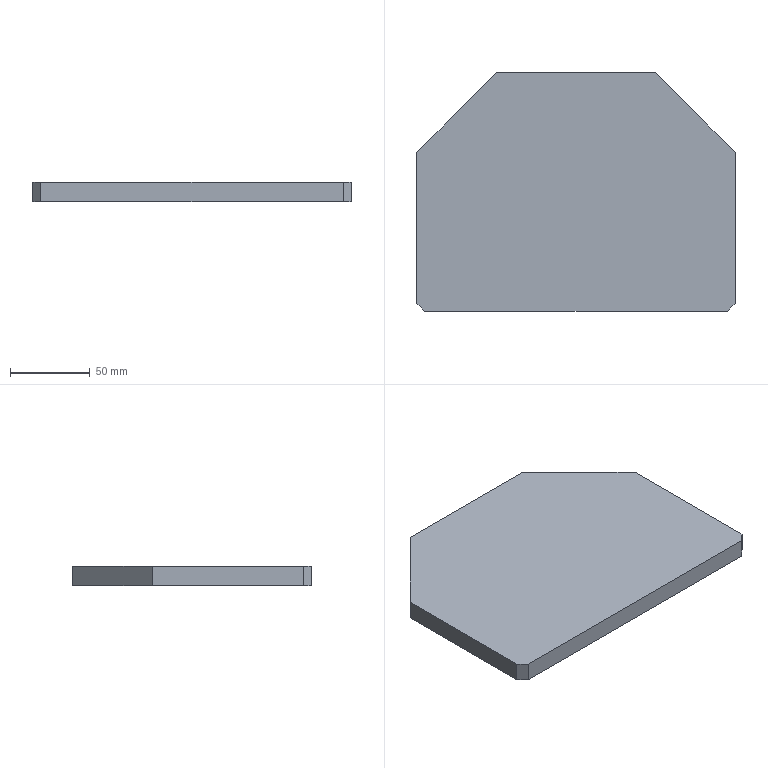Part | STEP file | [15] | 1 solid | 10 faces | box 200 x 150 x 12 mm | volume 329700 mm3 | plane 10
STEP:
#1=CARTESIAN_POINT('',(0.,0.,0.));
#2=DIRECTION('',(0.,0.,1.));
#3=DIRECTION('',(1.,0.,0.));
#4=AXIS2_PLACEMENT_3D('',#1,#2,#3);
#5=CARTESIAN_POINT('',(200.,5.,0.));
#6=VERTEX_POINT('',#5);
#7=CARTESIAN_POINT('',(200.,100.,0.));
#8=VERTEX_POINT('',#7);
#9=CARTESIAN_POINT('',(200.,75.,0.));
#10=DIRECTION('',(0.,1.,0.));
#11=VECTOR('',#10,1.);
#12=LINE('',#9,#11);
#13=CARTESIAN_POINT('',(100.,75.,0.));
#14=DIRECTION('',(0.,0.,-1.));
#15=DIRECTION('',(0.,-1.,0.));
#16=AXIS2_PLACEMENT_3D('',#13,#14,#15);
#17=PLANE('',#16);
#18=CARTESIAN_POINT('',(0.,-100.));
#19=DIRECTION('',(-1.,0.));
#20=VECTOR('',#19,1.);
#21=LINE('',#18,#20);
#22=(GEOMETRIC_REPRESENTATION_CONTEXT(2)PARAMETRIC_REPRESENTATION_CONTEXT()REPRESENTATION_CONTEXT('',''));
#23=DEFINITIONAL_REPRESENTATION('',(#21),#22);
#24=PCURVE('',#17,#23);
#25=CARTESIAN_POINT('',(200.,75.,12.));
#26=DIRECTION('',(1.,0.,0.));
#27=DIRECTION('',(0.,0.,1.));
#28=AXIS2_PLACEMENT_3D('',#25,#26,#27);
#29=PLANE('',#28);
#30=CARTESIAN_POINT('',(-12.,0.));
#31=DIRECTION('',(0.,-1.));
#32=VECTOR('',#31,1.);
#33=LINE('',#30,#32);
#34=(GEOMETRIC_REPRESENTATION_CONTEXT(2)PARAMETRIC_REPRESENTATION_CONTEXT()REPRESENTATION_CONTEXT('',''));
#35=DEFINITIONAL_REPRESENTATION('',(#33),#34);
#36=PCURVE('',#29,#35);
#37=SURFACE_CURVE('',#12,(#24,#36),.PCURVE_S1.);
#38=EDGE_CURVE('',#6,#8,#37,.T.);
#39=ORIENTED_EDGE('',*,*,#38,.F.);
#40=CARTESIAN_POINT('',(195.,0.,0.));
#41=VERTEX_POINT('',#40);
#42=CARTESIAN_POINT('',(185.,-10.,0.));
#43=DIRECTION('',(-0.7071,-0.7071,0.));
#44=VECTOR('',#43,1.);
#45=LINE('',#42,#44);
#46=CARTESIAN_POINT('',(85.,-85.));
#47=DIRECTION('',(0.7071,0.7071));
#48=VECTOR('',#47,1.);
#49=LINE('',#46,#48);
#50=(GEOMETRIC_REPRESENTATION_CONTEXT(2)PARAMETRIC_REPRESENTATION_CONTEXT()REPRESENTATION_CONTEXT('',''));
#51=DEFINITIONAL_REPRESENTATION('',(#49),#50);
#52=PCURVE('',#17,#51);
#53=CARTESIAN_POINT('',(200.,5.,12.));
#54=DIRECTION('',(-0.7071,0.7071,0.));
#55=DIRECTION('',(0.,0.,-1.));
#56=AXIS2_PLACEMENT_3D('',#53,#54,#55);
#57=PLANE('',#56);
#58=CARTESIAN_POINT('',(12.,21.213));
#59=DIRECTION('',(0.,1.));
#60=VECTOR('',#59,1.);
#61=LINE('',#58,#60);
#62=(GEOMETRIC_REPRESENTATION_CONTEXT(2)PARAMETRIC_REPRESENTATION_CONTEXT()REPRESENTATION_CONTEXT('',''));
#63=DEFINITIONAL_REPRESENTATION('',(#61),#62);
#64=PCURVE('',#57,#63);
#65=SURFACE_CURVE('',#45,(#52,#64),.PCURVE_S1.);
#66=EDGE_CURVE('',#6,#41,#65,.T.);
#67=ORIENTED_EDGE('',*,*,#66,.T.);
#68=CARTESIAN_POINT('',(5.,0.,0.));
#69=VERTEX_POINT('',#68);
#70=CARTESIAN_POINT('',(100.,0.,0.));
#71=DIRECTION('',(1.,0.,0.));
#72=VECTOR('',#71,1.);
#73=LINE('',#70,#72);
#74=CARTESIAN_POINT('',(75.,0.));
#75=DIRECTION('',(0.,-1.));
#76=VECTOR('',#75,1.);
#77=LINE('',#74,#76);
#78=(GEOMETRIC_REPRESENTATION_CONTEXT(2)PARAMETRIC_REPRESENTATION_CONTEXT()REPRESENTATION_CONTEXT('',''));
#79=DEFINITIONAL_REPRESENTATION('',(#77),#78);
#80=PCURVE('',#17,#79);
#81=CARTESIAN_POINT('',(100.,0.,12.));
#82=DIRECTION('',(0.,-1.,0.));
#83=DIRECTION('',(0.,0.,1.));
#84=AXIS2_PLACEMENT_3D('',#81,#82,#83);
#85=PLANE('',#84);
#86=CARTESIAN_POINT('',(-12.,0.));
#87=DIRECTION('',(0.,-1.));
#88=VECTOR('',#87,1.);
#89=LINE('',#86,#88);
#90=(GEOMETRIC_REPRESENTATION_CONTEXT(2)PARAMETRIC_REPRESENTATION_CONTEXT()REPRESENTATION_CONTEXT('',''));
#91=DEFINITIONAL_REPRESENTATION('',(#89),#90);
#92=PCURVE('',#85,#91);
#93=SURFACE_CURVE('',#73,(#80,#92),.PCURVE_S1.);
#94=EDGE_CURVE('',#69,#41,#93,.T.);
#95=ORIENTED_EDGE('',*,*,#94,.F.);
#96=CARTESIAN_POINT('',(0.,5.,0.));
#97=VERTEX_POINT('',#96);
#98=CARTESIAN_POINT('',(15.,-10.,0.));
#99=DIRECTION('',(-0.7071,0.7071,0.));
#100=VECTOR('',#99,1.);
#101=LINE('',#98,#100);
#102=CARTESIAN_POINT('',(85.,85.));
#103=DIRECTION('',(-0.7071,0.7071));
#104=VECTOR('',#103,1.);
#105=LINE('',#102,#104);
#106=(GEOMETRIC_REPRESENTATION_CONTEXT(2)PARAMETRIC_REPRESENTATION_CONTEXT()REPRESENTATION_CONTEXT('',''));
#107=DEFINITIONAL_REPRESENTATION('',(#105),#106);
#108=PCURVE('',#17,#107);
#109=CARTESIAN_POINT('',(5.,0.,12.));
#110=DIRECTION('',(0.7071,0.7071,0.));
#111=DIRECTION('',(0.,0.,-1.));
#112=AXIS2_PLACEMENT_3D('',#109,#110,#111);
#113=PLANE('',#112);
#114=CARTESIAN_POINT('',(12.,-14.142));
#115=DIRECTION('',(0.,1.));
#116=VECTOR('',#115,1.);
#117=LINE('',#114,#116);
#118=(GEOMETRIC_REPRESENTATION_CONTEXT(2)PARAMETRIC_REPRESENTATION_CONTEXT()REPRESENTATION_CONTEXT('',''));
#119=DEFINITIONAL_REPRESENTATION('',(#117),#118);
#120=PCURVE('',#113,#119);
#121=SURFACE_CURVE('',#101,(#108,#120),.PCURVE_S1.);
#122=EDGE_CURVE('',#69,#97,#121,.T.);
#123=ORIENTED_EDGE('',*,*,#122,.T.);
#124=CARTESIAN_POINT('',(0.,100.,0.));
#125=VERTEX_POINT('',#124);
#126=CARTESIAN_POINT('',(0.,75.,0.));
#127=DIRECTION('',(0.,-1.,0.));
#128=VECTOR('',#127,1.);
#129=LINE('',#126,#128);
#130=CARTESIAN_POINT('',(0.,100.));
#131=DIRECTION('',(1.,0.));
#132=VECTOR('',#131,1.);
#133=LINE('',#130,#132);
#134=(GEOMETRIC_REPRESENTATION_CONTEXT(2)PARAMETRIC_REPRESENTATION_CONTEXT()REPRESENTATION_CONTEXT('',''));
#135=DEFINITIONAL_REPRESENTATION('',(#133),#134);
#136=PCURVE('',#17,#135);
#137=CARTESIAN_POINT('',(0.,75.,12.));
#138=DIRECTION('',(-1.,0.,0.));
#139=DIRECTION('',(0.,0.,-1.));
#140=AXIS2_PLACEMENT_3D('',#137,#138,#139);
#141=PLANE('',#140);
#142=CARTESIAN_POINT('',(12.,0.));
#143=DIRECTION('',(0.,1.));
#144=VECTOR('',#143,1.);
#145=LINE('',#142,#144);
#146=(GEOMETRIC_REPRESENTATION_CONTEXT(2)PARAMETRIC_REPRESENTATION_CONTEXT()REPRESENTATION_CONTEXT('',''));
#147=DEFINITIONAL_REPRESENTATION('',(#145),#146);
#148=PCURVE('',#141,#147);
#149=SURFACE_CURVE('',#129,(#136,#148),.PCURVE_S1.);
#150=EDGE_CURVE('',#125,#97,#149,.T.);
#151=ORIENTED_EDGE('',*,*,#150,.F.);
#152=CARTESIAN_POINT('',(50.,150.,0.));
#153=VERTEX_POINT('',#152);
#154=CARTESIAN_POINT('',(37.5,137.5,0.));
#155=DIRECTION('',(0.7071,0.7071,0.));
#156=VECTOR('',#155,1.);
#157=LINE('',#154,#156);
#158=CARTESIAN_POINT('',(-62.5,62.5));
#159=DIRECTION('',(-0.7071,-0.7071));
#160=VECTOR('',#159,1.);
#161=LINE('',#158,#160);
#162=(GEOMETRIC_REPRESENTATION_CONTEXT(2)PARAMETRIC_REPRESENTATION_CONTEXT()REPRESENTATION_CONTEXT('',''));
#163=DEFINITIONAL_REPRESENTATION('',(#161),#162);
#164=PCURVE('',#17,#163);
#165=CARTESIAN_POINT('',(0.,100.,12.));
#166=DIRECTION('',(0.7071,-0.7071,0.));
#167=DIRECTION('',(0.,0.,-1.));
#168=AXIS2_PLACEMENT_3D('',#165,#166,#167);
#169=PLANE('',#168);
#170=CARTESIAN_POINT('',(12.,53.033));
#171=DIRECTION('',(0.,1.));
#172=VECTOR('',#171,1.);
#173=LINE('',#170,#172);
#174=(GEOMETRIC_REPRESENTATION_CONTEXT(2)PARAMETRIC_REPRESENTATION_CONTEXT()REPRESENTATION_CONTEXT('',''));
#175=DEFINITIONAL_REPRESENTATION('',(#173),#174);
#176=PCURVE('',#169,#175);
#177=SURFACE_CURVE('',#157,(#164,#176),.PCURVE_S1.);
#178=EDGE_CURVE('',#125,#153,#177,.T.);
#179=ORIENTED_EDGE('',*,*,#178,.T.);
#180=CARTESIAN_POINT('',(150.,150.,0.));
#181=VERTEX_POINT('',#180);
#182=CARTESIAN_POINT('',(100.,150.,0.));
#183=DIRECTION('',(-1.,0.,0.));
#184=VECTOR('',#183,1.);
#185=LINE('',#182,#184);
#186=CARTESIAN_POINT('',(-75.,0.));
#187=DIRECTION('',(0.,1.));
#188=VECTOR('',#187,1.);
#189=LINE('',#186,#188);
#190=(GEOMETRIC_REPRESENTATION_CONTEXT(2)PARAMETRIC_REPRESENTATION_CONTEXT()REPRESENTATION_CONTEXT('',''));
#191=DEFINITIONAL_REPRESENTATION('',(#189),#190);
#192=PCURVE('',#17,#191);
#193=CARTESIAN_POINT('',(100.,150.,12.));
#194=DIRECTION('',(0.,1.,0.));
#195=DIRECTION('',(0.,0.,-1.));
#196=AXIS2_PLACEMENT_3D('',#193,#194,#195);
#197=PLANE('',#196);
#198=CARTESIAN_POINT('',(12.,0.));
#199=DIRECTION('',(0.,1.));
#200=VECTOR('',#199,1.);
#201=LINE('',#198,#200);
#202=(GEOMETRIC_REPRESENTATION_CONTEXT(2)PARAMETRIC_REPRESENTATION_CONTEXT()REPRESENTATION_CONTEXT('',''));
#203=DEFINITIONAL_REPRESENTATION('',(#201),#202);
#204=PCURVE('',#197,#203);
#205=SURFACE_CURVE('',#185,(#192,#204),.PCURVE_S1.);
#206=EDGE_CURVE('',#181,#153,#205,.T.);
#207=ORIENTED_EDGE('',*,*,#206,.F.);
#208=CARTESIAN_POINT('',(162.5,137.5,0.));
#209=DIRECTION('',(0.7071,-0.7071,0.));
#210=VECTOR('',#209,1.);
#211=LINE('',#208,#210);
#212=CARTESIAN_POINT('',(-62.5,-62.5));
#213=DIRECTION('',(0.7071,-0.7071));
#214=VECTOR('',#213,1.);
#215=LINE('',#212,#214);
#216=(GEOMETRIC_REPRESENTATION_CONTEXT(2)PARAMETRIC_REPRESENTATION_CONTEXT()REPRESENTATION_CONTEXT('',''));
#217=DEFINITIONAL_REPRESENTATION('',(#215),#216);
#218=PCURVE('',#17,#217);
#219=CARTESIAN_POINT('',(150.,150.,12.));
#220=DIRECTION('',(-0.7071,-0.7071,0.));
#221=DIRECTION('',(0.,0.,-1.));
#222=AXIS2_PLACEMENT_3D('',#219,#220,#221);
#223=PLANE('',#222);
#224=CARTESIAN_POINT('',(12.,17.678));
#225=DIRECTION('',(0.,1.));
#226=VECTOR('',#225,1.);
#227=LINE('',#224,#226);
#228=(GEOMETRIC_REPRESENTATION_CONTEXT(2)PARAMETRIC_REPRESENTATION_CONTEXT()REPRESENTATION_CONTEXT('',''));
#229=DEFINITIONAL_REPRESENTATION('',(#227),#228);
#230=PCURVE('',#223,#229);
#231=SURFACE_CURVE('',#211,(#218,#230),.PCURVE_S1.);
#232=EDGE_CURVE('',#181,#8,#231,.T.);
#233=ORIENTED_EDGE('',*,*,#232,.T.);
#234=EDGE_LOOP('',(#39,#67,#95,#123,#151,#179,#207,#233));
#235=FACE_BOUND('',#234,.T.);
#236=ADVANCED_FACE('',(#235),#17,.T.);
#237=CARTESIAN_POINT('',(200.,100.,12.));
#238=VERTEX_POINT('',#237);
#239=CARTESIAN_POINT('',(200.,5.,12.));
#240=VERTEX_POINT('',#239);
#241=CARTESIAN_POINT('',(200.,75.,12.));
#242=DIRECTION('',(0.,-1.,0.));
#243=VECTOR('',#242,1.);
#244=LINE('',#241,#243);
#245=CARTESIAN_POINT('',(0.,0.));
#246=DIRECTION('',(0.,1.));
#247=VECTOR('',#246,1.);
#248=LINE('',#245,#247);
#249=(GEOMETRIC_REPRESENTATION_CONTEXT(2)PARAMETRIC_REPRESENTATION_CONTEXT()REPRESENTATION_CONTEXT('',''));
#250=DEFINITIONAL_REPRESENTATION('',(#248),#249);
#251=PCURVE('',#29,#250);
#252=CARTESIAN_POINT('',(100.,75.,12.));
#253=DIRECTION('',(0.,0.,1.));
#254=DIRECTION('',(0.,1.,0.));
#255=AXIS2_PLACEMENT_3D('',#252,#253,#254);
#256=PLANE('',#255);
#257=CARTESIAN_POINT('',(0.,-100.));
#258=DIRECTION('',(-1.,0.));
#259=VECTOR('',#258,1.);
#260=LINE('',#257,#259);
#261=(GEOMETRIC_REPRESENTATION_CONTEXT(2)PARAMETRIC_REPRESENTATION_CONTEXT()REPRESENTATION_CONTEXT('',''));
#262=DEFINITIONAL_REPRESENTATION('',(#260),#261);
#263=PCURVE('',#256,#262);
#264=SURFACE_CURVE('',#244,(#251,#263),.PCURVE_S1.);
#265=EDGE_CURVE('',#238,#240,#264,.T.);
#266=ORIENTED_EDGE('',*,*,#265,.T.);
#267=CARTESIAN_POINT('',(200.,5.,12.));
#268=DIRECTION('',(0.,0.,-1.));
#269=VECTOR('',#268,1.);
#270=LINE('',#267,#269);
#271=CARTESIAN_POINT('',(0.,70.));
#272=DIRECTION('',(-1.,0.));
#273=VECTOR('',#272,1.);
#274=LINE('',#271,#273);
#275=(GEOMETRIC_REPRESENTATION_CONTEXT(2)PARAMETRIC_REPRESENTATION_CONTEXT()REPRESENTATION_CONTEXT('',''));
#276=DEFINITIONAL_REPRESENTATION('',(#274),#275);
#277=PCURVE('',#29,#276);
#278=CARTESIAN_POINT('',(0.,0.));
#279=DIRECTION('',(1.,0.));
#280=VECTOR('',#279,1.);
#281=LINE('',#278,#280);
#282=(GEOMETRIC_REPRESENTATION_CONTEXT(2)PARAMETRIC_REPRESENTATION_CONTEXT()REPRESENTATION_CONTEXT('',''));
#283=DEFINITIONAL_REPRESENTATION('',(#281),#282);
#284=PCURVE('',#57,#283);
#285=SURFACE_CURVE('',#270,(#277,#284),.PCURVE_S1.);
#286=EDGE_CURVE('',#240,#6,#285,.T.);
#287=ORIENTED_EDGE('',*,*,#286,.T.);
#288=ORIENTED_EDGE('',*,*,#38,.T.);
#289=CARTESIAN_POINT('',(200.,100.,12.));
#290=DIRECTION('',(0.,0.,1.));
#291=VECTOR('',#290,1.);
#292=LINE('',#289,#291);
#293=CARTESIAN_POINT('',(0.,-25.));
#294=DIRECTION('',(1.,0.));
#295=VECTOR('',#294,1.);
#296=LINE('',#293,#295);
#297=(GEOMETRIC_REPRESENTATION_CONTEXT(2)PARAMETRIC_REPRESENTATION_CONTEXT()REPRESENTATION_CONTEXT('',''));
#298=DEFINITIONAL_REPRESENTATION('',(#296),#297);
#299=PCURVE('',#29,#298);
#300=CARTESIAN_POINT('',(0.,70.711));
#301=DIRECTION('',(-1.,0.));
#302=VECTOR('',#301,1.);
#303=LINE('',#300,#302);
#304=(GEOMETRIC_REPRESENTATION_CONTEXT(2)PARAMETRIC_REPRESENTATION_CONTEXT()REPRESENTATION_CONTEXT('',''));
#305=DEFINITIONAL_REPRESENTATION('',(#303),#304);
#306=PCURVE('',#223,#305);
#307=SURFACE_CURVE('',#292,(#299,#306),.PCURVE_S1.);
#308=EDGE_CURVE('',#8,#238,#307,.T.);
#309=ORIENTED_EDGE('',*,*,#308,.T.);
#310=EDGE_LOOP('',(#266,#287,#288,#309));
#311=FACE_BOUND('',#310,.T.);
#312=ADVANCED_FACE('',(#311),#29,.T.);
#313=ORIENTED_EDGE('',*,*,#206,.T.);
#314=CARTESIAN_POINT('',(50.,150.,12.));
#315=VERTEX_POINT('',#314);
#316=CARTESIAN_POINT('',(50.,150.,12.));
#317=DIRECTION('',(0.,0.,1.));
#318=VECTOR('',#317,1.);
#319=LINE('',#316,#318);
#320=CARTESIAN_POINT('',(0.,50.));
#321=DIRECTION('',(-1.,0.));
#322=VECTOR('',#321,1.);
#323=LINE('',#320,#322);
#324=(GEOMETRIC_REPRESENTATION_CONTEXT(2)PARAMETRIC_REPRESENTATION_CONTEXT()REPRESENTATION_CONTEXT('',''));
#325=DEFINITIONAL_REPRESENTATION('',(#323),#324);
#326=PCURVE('',#197,#325);
#327=CARTESIAN_POINT('',(0.,70.711));
#328=DIRECTION('',(-1.,0.));
#329=VECTOR('',#328,1.);
#330=LINE('',#327,#329);
#331=(GEOMETRIC_REPRESENTATION_CONTEXT(2)PARAMETRIC_REPRESENTATION_CONTEXT()REPRESENTATION_CONTEXT('',''));
#332=DEFINITIONAL_REPRESENTATION('',(#330),#331);
#333=PCURVE('',#169,#332);
#334=SURFACE_CURVE('',#319,(#326,#333),.PCURVE_S1.);
#335=EDGE_CURVE('',#153,#315,#334,.T.);
#336=ORIENTED_EDGE('',*,*,#335,.T.);
#337=CARTESIAN_POINT('',(150.,150.,12.));
#338=VERTEX_POINT('',#337);
#339=CARTESIAN_POINT('',(100.,150.,12.));
#340=DIRECTION('',(1.,0.,0.));
#341=VECTOR('',#340,1.);
#342=LINE('',#339,#341);
#343=CARTESIAN_POINT('',(0.,0.));
#344=DIRECTION('',(0.,-1.));
#345=VECTOR('',#344,1.);
#346=LINE('',#343,#345);
#347=(GEOMETRIC_REPRESENTATION_CONTEXT(2)PARAMETRIC_REPRESENTATION_CONTEXT()REPRESENTATION_CONTEXT('',''));
#348=DEFINITIONAL_REPRESENTATION('',(#346),#347);
#349=PCURVE('',#197,#348);
#350=CARTESIAN_POINT('',(75.,0.));
#351=DIRECTION('',(0.,-1.));
#352=VECTOR('',#351,1.);
#353=LINE('',#350,#352);
#354=(GEOMETRIC_REPRESENTATION_CONTEXT(2)PARAMETRIC_REPRESENTATION_CONTEXT()REPRESENTATION_CONTEXT('',''));
#355=DEFINITIONAL_REPRESENTATION('',(#353),#354);
#356=PCURVE('',#256,#355);
#357=SURFACE_CURVE('',#342,(#349,#356),.PCURVE_S1.);
#358=EDGE_CURVE('',#315,#338,#357,.T.);
#359=ORIENTED_EDGE('',*,*,#358,.T.);
#360=CARTESIAN_POINT('',(150.,150.,12.));
#361=DIRECTION('',(0.,0.,-1.));
#362=VECTOR('',#361,1.);
#363=LINE('',#360,#362);
#364=CARTESIAN_POINT('',(0.,-50.));
#365=DIRECTION('',(1.,0.));
#366=VECTOR('',#365,1.);
#367=LINE('',#364,#366);
#368=(GEOMETRIC_REPRESENTATION_CONTEXT(2)PARAMETRIC_REPRESENTATION_CONTEXT()REPRESENTATION_CONTEXT('',''));
#369=DEFINITIONAL_REPRESENTATION('',(#367),#368);
#370=PCURVE('',#197,#369);
#371=CARTESIAN_POINT('',(0.,0.));
#372=DIRECTION('',(1.,0.));
#373=VECTOR('',#372,1.);
#374=LINE('',#371,#373);
#375=(GEOMETRIC_REPRESENTATION_CONTEXT(2)PARAMETRIC_REPRESENTATION_CONTEXT()REPRESENTATION_CONTEXT('',''));
#376=DEFINITIONAL_REPRESENTATION('',(#374),#375);
#377=PCURVE('',#223,#376);
#378=SURFACE_CURVE('',#363,(#370,#377),.PCURVE_S1.);
#379=EDGE_CURVE('',#338,#181,#378,.T.);
#380=ORIENTED_EDGE('',*,*,#379,.T.);
#381=EDGE_LOOP('',(#313,#336,#359,#380));
#382=FACE_BOUND('',#381,.T.);
#383=ADVANCED_FACE('',(#382),#197,.T.);
#384=ORIENTED_EDGE('',*,*,#150,.T.);
#385=CARTESIAN_POINT('',(0.,5.,12.));
#386=VERTEX_POINT('',#385);
#387=CARTESIAN_POINT('',(0.,5.,12.));
#388=DIRECTION('',(0.,0.,1.));
#389=VECTOR('',#388,1.);
#390=LINE('',#387,#389);
#391=CARTESIAN_POINT('',(0.,70.));
#392=DIRECTION('',(-1.,0.));
#393=VECTOR('',#392,1.);
#394=LINE('',#391,#393);
#395=(GEOMETRIC_REPRESENTATION_CONTEXT(2)PARAMETRIC_REPRESENTATION_CONTEXT()REPRESENTATION_CONTEXT('',''));
#396=DEFINITIONAL_REPRESENTATION('',(#394),#395);
#397=PCURVE('',#141,#396);
#398=CARTESIAN_POINT('',(0.,7.071));
#399=DIRECTION('',(-1.,0.));
#400=VECTOR('',#399,1.);
#401=LINE('',#398,#400);
#402=(GEOMETRIC_REPRESENTATION_CONTEXT(2)PARAMETRIC_REPRESENTATION_CONTEXT()REPRESENTATION_CONTEXT('',''));
#403=DEFINITIONAL_REPRESENTATION('',(#401),#402);
#404=PCURVE('',#113,#403);
#405=SURFACE_CURVE('',#390,(#397,#404),.PCURVE_S1.);
#406=EDGE_CURVE('',#97,#386,#405,.T.);
#407=ORIENTED_EDGE('',*,*,#406,.T.);
#408=CARTESIAN_POINT('',(0.,100.,12.));
#409=VERTEX_POINT('',#408);
#410=CARTESIAN_POINT('',(0.,75.,12.));
#411=DIRECTION('',(0.,1.,0.));
#412=VECTOR('',#411,1.);
#413=LINE('',#410,#412);
#414=CARTESIAN_POINT('',(0.,0.));
#415=DIRECTION('',(0.,-1.));
#416=VECTOR('',#415,1.);
#417=LINE('',#414,#416);
#418=(GEOMETRIC_REPRESENTATION_CONTEXT(2)PARAMETRIC_REPRESENTATION_CONTEXT()REPRESENTATION_CONTEXT('',''));
#419=DEFINITIONAL_REPRESENTATION('',(#417),#418);
#420=PCURVE('',#141,#419);
#421=CARTESIAN_POINT('',(0.,100.));
#422=DIRECTION('',(1.,0.));
#423=VECTOR('',#422,1.);
#424=LINE('',#421,#423);
#425=(GEOMETRIC_REPRESENTATION_CONTEXT(2)PARAMETRIC_REPRESENTATION_CONTEXT()REPRESENTATION_CONTEXT('',''));
#426=DEFINITIONAL_REPRESENTATION('',(#424),#425);
#427=PCURVE('',#256,#426);
#428=SURFACE_CURVE('',#413,(#420,#427),.PCURVE_S1.);
#429=EDGE_CURVE('',#386,#409,#428,.T.);
#430=ORIENTED_EDGE('',*,*,#429,.T.);
#431=CARTESIAN_POINT('',(0.,100.,12.));
#432=DIRECTION('',(0.,0.,-1.));
#433=VECTOR('',#432,1.);
#434=LINE('',#431,#433);
#435=CARTESIAN_POINT('',(0.,-25.));
#436=DIRECTION('',(1.,0.));
#437=VECTOR('',#436,1.);
#438=LINE('',#435,#437);
#439=(GEOMETRIC_REPRESENTATION_CONTEXT(2)PARAMETRIC_REPRESENTATION_CONTEXT()REPRESENTATION_CONTEXT('',''));
#440=DEFINITIONAL_REPRESENTATION('',(#438),#439);
#441=PCURVE('',#141,#440);
#442=CARTESIAN_POINT('',(0.,0.));
#443=DIRECTION('',(1.,0.));
#444=VECTOR('',#443,1.);
#445=LINE('',#442,#444);
#446=(GEOMETRIC_REPRESENTATION_CONTEXT(2)PARAMETRIC_REPRESENTATION_CONTEXT()REPRESENTATION_CONTEXT('',''));
#447=DEFINITIONAL_REPRESENTATION('',(#445),#446);
#448=PCURVE('',#169,#447);
#449=SURFACE_CURVE('',#434,(#441,#448),.PCURVE_S1.);
#450=EDGE_CURVE('',#409,#125,#449,.T.);
#451=ORIENTED_EDGE('',*,*,#450,.T.);
#452=EDGE_LOOP('',(#384,#407,#430,#451));
#453=FACE_BOUND('',#452,.T.);
#454=ADVANCED_FACE('',(#453),#141,.T.);
#455=CARTESIAN_POINT('',(195.,0.,12.));
#456=VERTEX_POINT('',#455);
#457=CARTESIAN_POINT('',(5.,0.,12.));
#458=VERTEX_POINT('',#457);
#459=CARTESIAN_POINT('',(100.,0.,12.));
#460=DIRECTION('',(-1.,0.,0.));
#461=VECTOR('',#460,1.);
#462=LINE('',#459,#461);
#463=CARTESIAN_POINT('',(-75.,0.));
#464=DIRECTION('',(0.,1.));
#465=VECTOR('',#464,1.);
#466=LINE('',#463,#465);
#467=(GEOMETRIC_REPRESENTATION_CONTEXT(2)PARAMETRIC_REPRESENTATION_CONTEXT()REPRESENTATION_CONTEXT('',''));
#468=DEFINITIONAL_REPRESENTATION('',(#466),#467);
#469=PCURVE('',#256,#468);
#470=CARTESIAN_POINT('',(0.,0.));
#471=DIRECTION('',(0.,1.));
#472=VECTOR('',#471,1.);
#473=LINE('',#470,#472);
#474=(GEOMETRIC_REPRESENTATION_CONTEXT(2)PARAMETRIC_REPRESENTATION_CONTEXT()REPRESENTATION_CONTEXT('',''));
#475=DEFINITIONAL_REPRESENTATION('',(#473),#474);
#476=PCURVE('',#85,#475);
#477=SURFACE_CURVE('',#462,(#469,#476),.PCURVE_S1.);
#478=EDGE_CURVE('',#456,#458,#477,.T.);
#479=ORIENTED_EDGE('',*,*,#478,.F.);
#480=CARTESIAN_POINT('',(185.,-10.,12.));
#481=DIRECTION('',(0.7071,0.7071,0.));
#482=VECTOR('',#481,1.);
#483=LINE('',#480,#482);
#484=CARTESIAN_POINT('',(-85.,-85.));
#485=DIRECTION('',(0.7071,-0.7071));
#486=VECTOR('',#485,1.);
#487=LINE('',#484,#486);
#488=(GEOMETRIC_REPRESENTATION_CONTEXT(2)PARAMETRIC_REPRESENTATION_CONTEXT()REPRESENTATION_CONTEXT('',''));
#489=DEFINITIONAL_REPRESENTATION('',(#487),#488);
#490=PCURVE('',#256,#489);
#491=CARTESIAN_POINT('',(0.,21.213));
#492=DIRECTION('',(0.,-1.));
#493=VECTOR('',#492,1.);
#494=LINE('',#491,#493);
#495=(GEOMETRIC_REPRESENTATION_CONTEXT(2)PARAMETRIC_REPRESENTATION_CONTEXT()REPRESENTATION_CONTEXT('',''));
#496=DEFINITIONAL_REPRESENTATION('',(#494),#495);
#497=PCURVE('',#57,#496);
#498=SURFACE_CURVE('',#483,(#490,#497),.PCURVE_S1.);
#499=EDGE_CURVE('',#456,#240,#498,.T.);
#500=ORIENTED_EDGE('',*,*,#499,.T.);
#501=ORIENTED_EDGE('',*,*,#265,.F.);
#502=CARTESIAN_POINT('',(162.5,137.5,12.));
#503=DIRECTION('',(-0.7071,0.7071,0.));
#504=VECTOR('',#503,1.);
#505=LINE('',#502,#504);
#506=CARTESIAN_POINT('',(62.5,-62.5));
#507=DIRECTION('',(0.7071,0.7071));
#508=VECTOR('',#507,1.);
#509=LINE('',#506,#508);
#510=(GEOMETRIC_REPRESENTATION_CONTEXT(2)PARAMETRIC_REPRESENTATION_CONTEXT()REPRESENTATION_CONTEXT('',''));
#511=DEFINITIONAL_REPRESENTATION('',(#509),#510);
#512=PCURVE('',#256,#511);
#513=CARTESIAN_POINT('',(0.,17.678));
#514=DIRECTION('',(0.,-1.));
#515=VECTOR('',#514,1.);
#516=LINE('',#513,#515);
#517=(GEOMETRIC_REPRESENTATION_CONTEXT(2)PARAMETRIC_REPRESENTATION_CONTEXT()REPRESENTATION_CONTEXT('',''));
#518=DEFINITIONAL_REPRESENTATION('',(#516),#517);
#519=PCURVE('',#223,#518);
#520=SURFACE_CURVE('',#505,(#512,#519),.PCURVE_S1.);
#521=EDGE_CURVE('',#238,#338,#520,.T.);
#522=ORIENTED_EDGE('',*,*,#521,.T.);
#523=ORIENTED_EDGE('',*,*,#358,.F.);
#524=CARTESIAN_POINT('',(37.5,137.5,12.));
#525=DIRECTION('',(-0.7071,-0.7071,0.));
#526=VECTOR('',#525,1.);
#527=LINE('',#524,#526);
#528=CARTESIAN_POINT('',(62.5,62.5));
#529=DIRECTION('',(-0.7071,0.7071));
#530=VECTOR('',#529,1.);
#531=LINE('',#528,#530);
#532=(GEOMETRIC_REPRESENTATION_CONTEXT(2)PARAMETRIC_REPRESENTATION_CONTEXT()REPRESENTATION_CONTEXT('',''));
#533=DEFINITIONAL_REPRESENTATION('',(#531),#532);
#534=PCURVE('',#256,#533);
#535=CARTESIAN_POINT('',(0.,53.033));
#536=DIRECTION('',(0.,-1.));
#537=VECTOR('',#536,1.);
#538=LINE('',#535,#537);
#539=(GEOMETRIC_REPRESENTATION_CONTEXT(2)PARAMETRIC_REPRESENTATION_CONTEXT()REPRESENTATION_CONTEXT('',''));
#540=DEFINITIONAL_REPRESENTATION('',(#538),#539);
#541=PCURVE('',#169,#540);
#542=SURFACE_CURVE('',#527,(#534,#541),.PCURVE_S1.);
#543=EDGE_CURVE('',#315,#409,#542,.T.);
#544=ORIENTED_EDGE('',*,*,#543,.T.);
#545=ORIENTED_EDGE('',*,*,#429,.F.);
#546=CARTESIAN_POINT('',(15.,-10.,12.));
#547=DIRECTION('',(0.7071,-0.7071,0.));
#548=VECTOR('',#547,1.);
#549=LINE('',#546,#548);
#550=CARTESIAN_POINT('',(-85.,85.));
#551=DIRECTION('',(-0.7071,-0.7071));
#552=VECTOR('',#551,1.);
#553=LINE('',#550,#552);
#554=(GEOMETRIC_REPRESENTATION_CONTEXT(2)PARAMETRIC_REPRESENTATION_CONTEXT()REPRESENTATION_CONTEXT('',''));
#555=DEFINITIONAL_REPRESENTATION('',(#553),#554);
#556=PCURVE('',#256,#555);
#557=CARTESIAN_POINT('',(0.,-14.142));
#558=DIRECTION('',(0.,-1.));
#559=VECTOR('',#558,1.);
#560=LINE('',#557,#559);
#561=(GEOMETRIC_REPRESENTATION_CONTEXT(2)PARAMETRIC_REPRESENTATION_CONTEXT()REPRESENTATION_CONTEXT('',''));
#562=DEFINITIONAL_REPRESENTATION('',(#560),#561);
#563=PCURVE('',#113,#562);
#564=SURFACE_CURVE('',#549,(#556,#563),.PCURVE_S1.);
#565=EDGE_CURVE('',#386,#458,#564,.T.);
#566=ORIENTED_EDGE('',*,*,#565,.T.);
#567=EDGE_LOOP('',(#479,#500,#501,#522,#523,#544,#545,#566));
#568=FACE_BOUND('',#567,.T.);
#569=ADVANCED_FACE('',(#568),#256,.T.);
#570=ORIENTED_EDGE('',*,*,#94,.T.);
#571=CARTESIAN_POINT('',(195.,0.,12.));
#572=DIRECTION('',(0.,0.,1.));
#573=VECTOR('',#572,1.);
#574=LINE('',#571,#573);
#575=CARTESIAN_POINT('',(0.,-95.));
#576=DIRECTION('',(1.,0.));
#577=VECTOR('',#576,1.);
#578=LINE('',#575,#577);
#579=(GEOMETRIC_REPRESENTATION_CONTEXT(2)PARAMETRIC_REPRESENTATION_CONTEXT()REPRESENTATION_CONTEXT('',''));
#580=DEFINITIONAL_REPRESENTATION('',(#578),#579);
#581=PCURVE('',#85,#580);
#582=CARTESIAN_POINT('',(0.,7.071));
#583=DIRECTION('',(-1.,0.));
#584=VECTOR('',#583,1.);
#585=LINE('',#582,#584);
#586=(GEOMETRIC_REPRESENTATION_CONTEXT(2)PARAMETRIC_REPRESENTATION_CONTEXT()REPRESENTATION_CONTEXT('',''));
#587=DEFINITIONAL_REPRESENTATION('',(#585),#586);
#588=PCURVE('',#57,#587);
#589=SURFACE_CURVE('',#574,(#581,#588),.PCURVE_S1.);
#590=EDGE_CURVE('',#41,#456,#589,.T.);
#591=ORIENTED_EDGE('',*,*,#590,.T.);
#592=ORIENTED_EDGE('',*,*,#478,.T.);
#593=CARTESIAN_POINT('',(5.,0.,12.));
#594=DIRECTION('',(0.,0.,-1.));
#595=VECTOR('',#594,1.);
#596=LINE('',#593,#595);
#597=CARTESIAN_POINT('',(0.,95.));
#598=DIRECTION('',(-1.,0.));
#599=VECTOR('',#598,1.);
#600=LINE('',#597,#599);
#601=(GEOMETRIC_REPRESENTATION_CONTEXT(2)PARAMETRIC_REPRESENTATION_CONTEXT()REPRESENTATION_CONTEXT('',''));
#602=DEFINITIONAL_REPRESENTATION('',(#600),#601);
#603=PCURVE('',#85,#602);
#604=CARTESIAN_POINT('',(0.,0.));
#605=DIRECTION('',(1.,0.));
#606=VECTOR('',#605,1.);
#607=LINE('',#604,#606);
#608=(GEOMETRIC_REPRESENTATION_CONTEXT(2)PARAMETRIC_REPRESENTATION_CONTEXT()REPRESENTATION_CONTEXT('',''));
#609=DEFINITIONAL_REPRESENTATION('',(#607),#608);
#610=PCURVE('',#113,#609);
#611=SURFACE_CURVE('',#596,(#603,#610),.PCURVE_S1.);
#612=EDGE_CURVE('',#458,#69,#611,.T.);
#613=ORIENTED_EDGE('',*,*,#612,.T.);
#614=EDGE_LOOP('',(#570,#591,#592,#613));
#615=FACE_BOUND('',#614,.T.);
#616=ADVANCED_FACE('',(#615),#85,.T.);
#617=ORIENTED_EDGE('',*,*,#521,.F.);
#618=ORIENTED_EDGE('',*,*,#308,.F.);
#619=ORIENTED_EDGE('',*,*,#232,.F.);
#620=ORIENTED_EDGE('',*,*,#379,.F.);
#621=EDGE_LOOP('',(#617,#618,#619,#620));
#622=FACE_BOUND('',#621,.T.);
#623=ADVANCED_FACE('',(#622),#223,.F.);
#624=ORIENTED_EDGE('',*,*,#543,.F.);
#625=ORIENTED_EDGE('',*,*,#335,.F.);
#626=ORIENTED_EDGE('',*,*,#178,.F.);
#627=ORIENTED_EDGE('',*,*,#450,.F.);
#628=EDGE_LOOP('',(#624,#625,#626,#627));
#629=FACE_BOUND('',#628,.T.);
#630=ADVANCED_FACE('',(#629),#169,.F.);
#631=ORIENTED_EDGE('',*,*,#565,.F.);
#632=ORIENTED_EDGE('',*,*,#406,.F.);
#633=ORIENTED_EDGE('',*,*,#122,.F.);
#634=ORIENTED_EDGE('',*,*,#612,.F.);
#635=EDGE_LOOP('',(#631,#632,#633,#634));
#636=FACE_BOUND('',#635,.T.);
#637=ADVANCED_FACE('',(#636),#113,.F.);
#638=ORIENTED_EDGE('',*,*,#499,.F.);
#639=ORIENTED_EDGE('',*,*,#590,.F.);
#640=ORIENTED_EDGE('',*,*,#66,.F.);
#641=ORIENTED_EDGE('',*,*,#286,.F.);
#642=EDGE_LOOP('',(#638,#639,#640,#641));
#643=FACE_BOUND('',#642,.T.);
#644=ADVANCED_FACE('',(#643),#57,.F.);
#645=CLOSED_SHELL('',(#236,#312,#383,#454,#569,#616,#623,#630,#637,#644));
#646=MANIFOLD_SOLID_BREP('',#645);
#647=(LENGTH_UNIT()NAMED_UNIT(*)SI_UNIT(.MILLI.,.METRE.));
#648=UNCERTAINTY_MEASURE_WITH_UNIT(LENGTH_MEASURE(0.0000001),#647,'','');
#649=(NAMED_UNIT(*)PLANE_ANGLE_UNIT()SI_UNIT($,.RADIAN.));
#650=(NAMED_UNIT(*)SI_UNIT($,.STERADIAN.)SOLID_ANGLE_UNIT());
#651=(GEOMETRIC_REPRESENTATION_CONTEXT(3)GLOBAL_UNCERTAINTY_ASSIGNED_CONTEXT((#648))GLOBAL_UNIT_ASSIGNED_CONTEXT((#647,#649,#650))REPRESENTATION_CONTEXT('',''));
#652=ADVANCED_BREP_SHAPE_REPRESENTATION('',(#4,#646),#651);